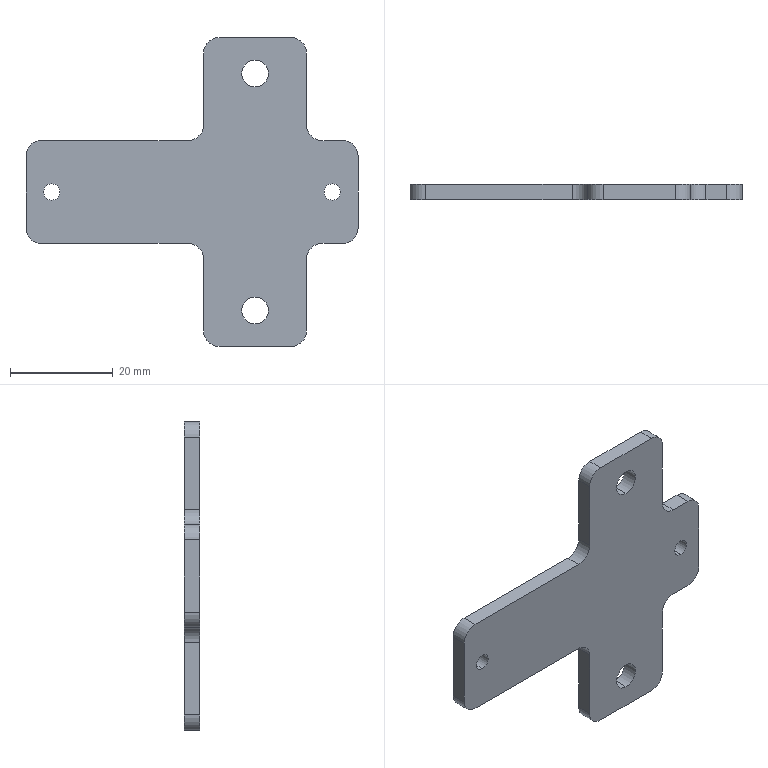Part | SolidWorks | features BaseBody 1 | 1 solid | 34 faces | box 64.5 x 3 x 60 mm | volume 6071 mm3 | cylinder 20 | plane 14 | commonest cylinder face diameters 6 x12 3.2 x4 5.2 x4
STEP:
#1=CARTESIAN_POINT('',(25.,0.,-31.6));
#2=VERTEX_POINT('',#1);
#3=CARTESIAN_POINT('',(25.,0.,-28.4));
#4=VERTEX_POINT('',#3);
#5=CARTESIAN_POINT('',(25.,0.,-30.));
#6=DIRECTION('',(0.,1.,0.));
#7=DIRECTION('',(0.,0.,1.));
#8=AXIS2_PLACEMENT_3D('',#5,#6,#7);
#9=CIRCLE('',#8,1.6);
#10=EDGE_CURVE('',#2,#4,#9,.T.);
#11=ORIENTED_EDGE('',*,*,#10,.F.);
#12=CARTESIAN_POINT('',(25.,3.,-31.6));
#13=VERTEX_POINT('',#12);
#14=CARTESIAN_POINT('',(25.,-39.878,-31.6));
#15=DIRECTION('',(0.,1.,0.));
#16=VECTOR('',#15,1000.);
#17=LINE('',#14,#16);
#18=EDGE_CURVE('',#2,#13,#17,.T.);
#19=ORIENTED_EDGE('',*,*,#18,.T.);
#20=CARTESIAN_POINT('',(25.,3.,-28.4));
#21=VERTEX_POINT('',#20);
#22=CARTESIAN_POINT('',(25.,3.,-30.));
#23=DIRECTION('',(0.,1.,0.));
#24=DIRECTION('',(0.,0.,1.));
#25=AXIS2_PLACEMENT_3D('',#22,#23,#24);
#26=CIRCLE('',#25,1.6);
#27=EDGE_CURVE('',#13,#21,#26,.T.);
#28=ORIENTED_EDGE('',*,*,#27,.T.);
#29=CARTESIAN_POINT('',(25.,-39.878,-28.4));
#30=DIRECTION('',(0.,1.,0.));
#31=VECTOR('',#30,1000.);
#32=LINE('',#29,#31);
#33=EDGE_CURVE('',#4,#21,#32,.T.);
#34=ORIENTED_EDGE('',*,*,#33,.F.);
#35=EDGE_LOOP('',(#11,#19,#28,#34));
#36=FACE_OUTER_BOUND('',#35,.T.);
#37=CARTESIAN_POINT('',(25.,-39.878,-30.));
#38=DIRECTION('',(0.,1.,0.));
#39=DIRECTION('',(0.,0.,1.));
#40=AXIS2_PLACEMENT_3D('',#37,#38,#39);
#41=CYLINDRICAL_SURFACE('',#40,1.6);
#42=ADVANCED_FACE('',(#36),#41,.F.);
#43=CARTESIAN_POINT('',(-29.5,0.,-31.6));
#44=VERTEX_POINT('',#43);
#45=CARTESIAN_POINT('',(-29.5,0.,-28.4));
#46=VERTEX_POINT('',#45);
#47=CARTESIAN_POINT('',(-29.5,0.,-30.));
#48=DIRECTION('',(0.,1.,0.));
#49=DIRECTION('',(0.,0.,1.));
#50=AXIS2_PLACEMENT_3D('',#47,#48,#49);
#51=CIRCLE('',#50,1.6);
#52=EDGE_CURVE('',#44,#46,#51,.T.);
#53=ORIENTED_EDGE('',*,*,#52,.F.);
#54=CARTESIAN_POINT('',(-29.5,3.,-31.6));
#55=VERTEX_POINT('',#54);
#56=CARTESIAN_POINT('',(-29.5,-39.878,-31.6));
#57=DIRECTION('',(0.,1.,0.));
#58=VECTOR('',#57,1000.);
#59=LINE('',#56,#58);
#60=EDGE_CURVE('',#44,#55,#59,.T.);
#61=ORIENTED_EDGE('',*,*,#60,.T.);
#62=CARTESIAN_POINT('',(-29.5,3.,-28.4));
#63=VERTEX_POINT('',#62);
#64=CARTESIAN_POINT('',(-29.5,3.,-30.));
#65=DIRECTION('',(0.,1.,0.));
#66=DIRECTION('',(0.,0.,1.));
#67=AXIS2_PLACEMENT_3D('',#64,#65,#66);
#68=CIRCLE('',#67,1.6);
#69=EDGE_CURVE('',#55,#63,#68,.T.);
#70=ORIENTED_EDGE('',*,*,#69,.T.);
#71=CARTESIAN_POINT('',(-29.5,-39.878,-28.4));
#72=DIRECTION('',(0.,1.,0.));
#73=VECTOR('',#72,1000.);
#74=LINE('',#71,#73);
#75=EDGE_CURVE('',#46,#63,#74,.T.);
#76=ORIENTED_EDGE('',*,*,#75,.F.);
#77=EDGE_LOOP('',(#53,#61,#70,#76));
#78=FACE_OUTER_BOUND('',#77,.T.);
#79=CARTESIAN_POINT('',(-29.5,-39.878,-30.));
#80=DIRECTION('',(0.,1.,0.));
#81=DIRECTION('',(0.,0.,1.));
#82=AXIS2_PLACEMENT_3D('',#79,#80,#81);
#83=CYLINDRICAL_SURFACE('',#82,1.6);
#84=ADVANCED_FACE('',(#78),#83,.F.);
#85=CARTESIAN_POINT('',(10.,3.,-55.6));
#86=VERTEX_POINT('',#85);
#87=CARTESIAN_POINT('',(10.,3.,-50.4));
#88=VERTEX_POINT('',#87);
#89=CARTESIAN_POINT('',(10.,3.,-53.));
#90=DIRECTION('',(0.,1.,0.));
#91=DIRECTION('',(0.,0.,-1.));
#92=AXIS2_PLACEMENT_3D('',#89,#90,#91);
#93=CIRCLE('',#92,2.6);
#94=EDGE_CURVE('',#86,#88,#93,.T.);
#95=ORIENTED_EDGE('',*,*,#94,.T.);
#96=CARTESIAN_POINT('',(10.,0.,-50.4));
#97=VERTEX_POINT('',#96);
#98=CARTESIAN_POINT('',(10.,3.,-50.4));
#99=DIRECTION('',(0.,-1.,0.));
#100=VECTOR('',#99,1000.);
#101=LINE('',#98,#100);
#102=EDGE_CURVE('',#88,#97,#101,.T.);
#103=ORIENTED_EDGE('',*,*,#102,.T.);
#104=CARTESIAN_POINT('',(10.,0.,-55.6));
#105=VERTEX_POINT('',#104);
#106=CARTESIAN_POINT('',(10.,0.,-53.));
#107=DIRECTION('',(0.,1.,0.));
#108=DIRECTION('',(0.,0.,-1.));
#109=AXIS2_PLACEMENT_3D('',#106,#107,#108);
#110=CIRCLE('',#109,2.6);
#111=EDGE_CURVE('',#105,#97,#110,.T.);
#112=ORIENTED_EDGE('',*,*,#111,.F.);
#113=CARTESIAN_POINT('',(10.,3.,-55.6));
#114=DIRECTION('',(0.,-1.,0.));
#115=VECTOR('',#114,1000.);
#116=LINE('',#113,#115);
#117=EDGE_CURVE('',#86,#105,#116,.T.);
#118=ORIENTED_EDGE('',*,*,#117,.F.);
#119=EDGE_LOOP('',(#95,#103,#112,#118));
#120=FACE_OUTER_BOUND('',#119,.T.);
#121=CARTESIAN_POINT('',(10.,3.,-53.));
#122=DIRECTION('',(0.,-1.,0.));
#123=DIRECTION('',(0.,0.,-1.));
#124=AXIS2_PLACEMENT_3D('',#121,#122,#123);
#125=CYLINDRICAL_SURFACE('',#124,2.6);
#126=ADVANCED_FACE('',(#120),#125,.F.);
#127=CARTESIAN_POINT('',(10.,3.,-9.6));
#128=VERTEX_POINT('',#127);
#129=CARTESIAN_POINT('',(10.,3.,-4.4));
#130=VERTEX_POINT('',#129);
#131=CARTESIAN_POINT('',(10.,3.,-7.));
#132=DIRECTION('',(0.,1.,0.));
#133=DIRECTION('',(0.,0.,-1.));
#134=AXIS2_PLACEMENT_3D('',#131,#132,#133);
#135=CIRCLE('',#134,2.6);
#136=EDGE_CURVE('',#128,#130,#135,.T.);
#137=ORIENTED_EDGE('',*,*,#136,.T.);
#138=CARTESIAN_POINT('',(10.,0.,-4.4));
#139=VERTEX_POINT('',#138);
#140=CARTESIAN_POINT('',(10.,3.,-4.4));
#141=DIRECTION('',(0.,-1.,0.));
#142=VECTOR('',#141,1000.);
#143=LINE('',#140,#142);
#144=EDGE_CURVE('',#130,#139,#143,.T.);
#145=ORIENTED_EDGE('',*,*,#144,.T.);
#146=CARTESIAN_POINT('',(10.,0.,-9.6));
#147=VERTEX_POINT('',#146);
#148=CARTESIAN_POINT('',(10.,0.,-7.));
#149=DIRECTION('',(0.,1.,0.));
#150=DIRECTION('',(0.,0.,-1.));
#151=AXIS2_PLACEMENT_3D('',#148,#149,#150);
#152=CIRCLE('',#151,2.6);
#153=EDGE_CURVE('',#147,#139,#152,.T.);
#154=ORIENTED_EDGE('',*,*,#153,.F.);
#155=CARTESIAN_POINT('',(10.,3.,-9.6));
#156=DIRECTION('',(0.,-1.,0.));
#157=VECTOR('',#156,1000.);
#158=LINE('',#155,#157);
#159=EDGE_CURVE('',#128,#147,#158,.T.);
#160=ORIENTED_EDGE('',*,*,#159,.F.);
#161=EDGE_LOOP('',(#137,#145,#154,#160));
#162=FACE_OUTER_BOUND('',#161,.T.);
#163=CARTESIAN_POINT('',(10.,3.,-7.));
#164=DIRECTION('',(0.,-1.,0.));
#165=DIRECTION('',(0.,0.,-1.));
#166=AXIS2_PLACEMENT_3D('',#163,#164,#165);
#167=CYLINDRICAL_SURFACE('',#166,2.6);
#168=ADVANCED_FACE('',(#162),#167,.F.);
#169=CARTESIAN_POINT('',(25.,3.,-30.));
#170=DIRECTION('',(0.,1.,0.));
#171=DIRECTION('',(0.,0.,1.));
#172=AXIS2_PLACEMENT_3D('',#169,#170,#171);
#173=CIRCLE('',#172,1.6);
#174=EDGE_CURVE('',#21,#13,#173,.T.);
#175=ORIENTED_EDGE('',*,*,#174,.F.);
#176=ORIENTED_EDGE('',*,*,#27,.F.);
#177=EDGE_LOOP('',(#175,#176));
#178=FACE_BOUND('',#177,.T.);
#179=CARTESIAN_POINT('',(-29.5,3.,-30.));
#180=DIRECTION('',(0.,1.,0.));
#181=DIRECTION('',(0.,0.,1.));
#182=AXIS2_PLACEMENT_3D('',#179,#180,#181);
#183=CIRCLE('',#182,1.6);
#184=EDGE_CURVE('',#63,#55,#183,.T.);
#185=ORIENTED_EDGE('',*,*,#184,.F.);
#186=ORIENTED_EDGE('',*,*,#69,.F.);
#187=EDGE_LOOP('',(#185,#186));
#188=FACE_BOUND('',#187,.T.);
#189=ORIENTED_EDGE('',*,*,#94,.F.);
#190=CARTESIAN_POINT('',(10.,3.,-53.));
#191=DIRECTION('',(0.,1.,0.));
#192=DIRECTION('',(0.,0.,-1.));
#193=AXIS2_PLACEMENT_3D('',#190,#191,#192);
#194=CIRCLE('',#193,2.6);
#195=EDGE_CURVE('',#88,#86,#194,.T.);
#196=ORIENTED_EDGE('',*,*,#195,.F.);
#197=EDGE_LOOP('',(#189,#196));
#198=FACE_BOUND('',#197,.T.);
#199=ORIENTED_EDGE('',*,*,#136,.F.);
#200=CARTESIAN_POINT('',(10.,3.,-7.));
#201=DIRECTION('',(0.,1.,0.));
#202=DIRECTION('',(0.,0.,-1.));
#203=AXIS2_PLACEMENT_3D('',#200,#201,#202);
#204=CIRCLE('',#203,2.6);
#205=EDGE_CURVE('',#130,#128,#204,.T.);
#206=ORIENTED_EDGE('',*,*,#205,.F.);
#207=EDGE_LOOP('',(#199,#206));
#208=FACE_BOUND('',#207,.T.);
#209=CARTESIAN_POINT('',(-31.5,3.,-20.));
#210=VERTEX_POINT('',#209);
#211=CARTESIAN_POINT('',(-34.5,3.,-23.));
#212=VERTEX_POINT('',#211);
#213=CARTESIAN_POINT('',(-31.5,3.,-23.));
#214=DIRECTION('',(0.,-1.,0.));
#215=DIRECTION('',(0.,0.,1.));
#216=AXIS2_PLACEMENT_3D('',#213,#214,#215);
#217=CIRCLE('',#216,3.);
#218=EDGE_CURVE('',#210,#212,#217,.T.);
#219=ORIENTED_EDGE('',*,*,#218,.F.);
#220=CARTESIAN_POINT('',(-3.,3.,-20.));
#221=VERTEX_POINT('',#220);
#222=CARTESIAN_POINT('',(0.,3.,-20.));
#223=DIRECTION('',(-1.,0.,0.));
#224=VECTOR('',#223,1000.);
#225=LINE('',#222,#224);
#226=EDGE_CURVE('',#221,#210,#225,.T.);
#227=ORIENTED_EDGE('',*,*,#226,.F.);
#228=CARTESIAN_POINT('',(0.,3.,-17.));
#229=VERTEX_POINT('',#228);
#230=CARTESIAN_POINT('',(-3.,3.,-17.));
#231=DIRECTION('',(0.,1.,0.));
#232=DIRECTION('',(0.,0.,1.));
#233=AXIS2_PLACEMENT_3D('',#230,#231,#232);
#234=CIRCLE('',#233,3.);
#235=EDGE_CURVE('',#229,#221,#234,.T.);
#236=ORIENTED_EDGE('',*,*,#235,.F.);
#237=CARTESIAN_POINT('',(0.,3.,-3.));
#238=VERTEX_POINT('',#237);
#239=CARTESIAN_POINT('',(0.,3.,0.));
#240=DIRECTION('',(0.,0.,-1.));
#241=VECTOR('',#240,1000.);
#242=LINE('',#239,#241);
#243=EDGE_CURVE('',#238,#229,#242,.T.);
#244=ORIENTED_EDGE('',*,*,#243,.F.);
#245=CARTESIAN_POINT('',(3.,3.,0.));
#246=VERTEX_POINT('',#245);
#247=CARTESIAN_POINT('',(3.,3.,-3.));
#248=DIRECTION('',(0.,-1.,0.));
#249=DIRECTION('',(0.,0.,-1.));
#250=AXIS2_PLACEMENT_3D('',#247,#248,#249);
#251=CIRCLE('',#250,3.);
#252=EDGE_CURVE('',#246,#238,#251,.T.);
#253=ORIENTED_EDGE('',*,*,#252,.F.);
#254=CARTESIAN_POINT('',(17.,3.,0.));
#255=VERTEX_POINT('',#254);
#256=CARTESIAN_POINT('',(0.,3.,0.));
#257=DIRECTION('',(-1.,0.,0.));
#258=VECTOR('',#257,1000.);
#259=LINE('',#256,#258);
#260=EDGE_CURVE('',#255,#246,#259,.T.);
#261=ORIENTED_EDGE('',*,*,#260,.F.);
#262=CARTESIAN_POINT('',(20.,3.,-3.));
#263=VERTEX_POINT('',#262);
#264=CARTESIAN_POINT('',(17.,3.,-3.));
#265=DIRECTION('',(0.,-1.,0.));
#266=DIRECTION('',(0.,0.,-1.));
#267=AXIS2_PLACEMENT_3D('',#264,#265,#266);
#268=CIRCLE('',#267,3.);
#269=EDGE_CURVE('',#263,#255,#268,.T.);
#270=ORIENTED_EDGE('',*,*,#269,.F.);
#271=CARTESIAN_POINT('',(20.,3.,-17.));
#272=VERTEX_POINT('',#271);
#273=CARTESIAN_POINT('',(20.,3.,0.));
#274=DIRECTION('',(0.,0.,1.));
#275=VECTOR('',#274,1000.);
#276=LINE('',#273,#275);
#277=EDGE_CURVE('',#272,#263,#276,.T.);
#278=ORIENTED_EDGE('',*,*,#277,.F.);
#279=CARTESIAN_POINT('',(23.,3.,-20.));
#280=VERTEX_POINT('',#279);
#281=CARTESIAN_POINT('',(23.,3.,-17.));
#282=DIRECTION('',(0.,1.,0.));
#283=DIRECTION('',(0.,0.,1.));
#284=AXIS2_PLACEMENT_3D('',#281,#282,#283);
#285=CIRCLE('',#284,3.);
#286=EDGE_CURVE('',#280,#272,#285,.T.);
#287=ORIENTED_EDGE('',*,*,#286,.F.);
#288=CARTESIAN_POINT('',(27.,3.,-20.));
#289=VERTEX_POINT('',#288);
#290=CARTESIAN_POINT('',(0.,3.,-20.));
#291=DIRECTION('',(-1.,0.,0.));
#292=VECTOR('',#291,1000.);
#293=LINE('',#290,#292);
#294=EDGE_CURVE('',#289,#280,#293,.T.);
#295=ORIENTED_EDGE('',*,*,#294,.F.);
#296=CARTESIAN_POINT('',(30.,3.,-23.));
#297=VERTEX_POINT('',#296);
#298=CARTESIAN_POINT('',(27.,3.,-23.));
#299=DIRECTION('',(0.,-1.,0.));
#300=DIRECTION('',(0.,0.,1.));
#301=AXIS2_PLACEMENT_3D('',#298,#299,#300);
#302=CIRCLE('',#301,3.);
#303=EDGE_CURVE('',#297,#289,#302,.T.);
#304=ORIENTED_EDGE('',*,*,#303,.F.);
#305=CARTESIAN_POINT('',(30.,3.,-37.));
#306=VERTEX_POINT('',#305);
#307=CARTESIAN_POINT('',(30.,3.,0.));
#308=DIRECTION('',(0.,0.,1.));
#309=VECTOR('',#308,1000.);
#310=LINE('',#307,#309);
#311=EDGE_CURVE('',#306,#297,#310,.T.);
#312=ORIENTED_EDGE('',*,*,#311,.F.);
#313=CARTESIAN_POINT('',(27.,3.,-40.));
#314=VERTEX_POINT('',#313);
#315=CARTESIAN_POINT('',(27.,3.,-37.));
#316=DIRECTION('',(0.,-1.,0.));
#317=DIRECTION('',(0.,0.,1.));
#318=AXIS2_PLACEMENT_3D('',#315,#316,#317);
#319=CIRCLE('',#318,3.);
#320=EDGE_CURVE('',#314,#306,#319,.T.);
#321=ORIENTED_EDGE('',*,*,#320,.F.);
#322=CARTESIAN_POINT('',(23.,3.,-40.));
#323=VERTEX_POINT('',#322);
#324=CARTESIAN_POINT('',(0.,3.,-40.));
#325=DIRECTION('',(1.,0.,0.));
#326=VECTOR('',#325,1000.);
#327=LINE('',#324,#326);
#328=EDGE_CURVE('',#323,#314,#327,.T.);
#329=ORIENTED_EDGE('',*,*,#328,.F.);
#330=CARTESIAN_POINT('',(20.,3.,-43.));
#331=VERTEX_POINT('',#330);
#332=CARTESIAN_POINT('',(23.,3.,-43.));
#333=DIRECTION('',(0.,1.,0.));
#334=DIRECTION('',(0.,0.,1.));
#335=AXIS2_PLACEMENT_3D('',#332,#333,#334);
#336=CIRCLE('',#335,3.);
#337=EDGE_CURVE('',#331,#323,#336,.T.);
#338=ORIENTED_EDGE('',*,*,#337,.F.);
#339=CARTESIAN_POINT('',(20.,3.,-57.));
#340=VERTEX_POINT('',#339);
#341=CARTESIAN_POINT('',(20.,3.,0.));
#342=DIRECTION('',(0.,0.,1.));
#343=VECTOR('',#342,1000.);
#344=LINE('',#341,#343);
#345=EDGE_CURVE('',#340,#331,#344,.T.);
#346=ORIENTED_EDGE('',*,*,#345,.F.);
#347=CARTESIAN_POINT('',(17.,3.,-60.));
#348=VERTEX_POINT('',#347);
#349=CARTESIAN_POINT('',(17.,3.,-57.));
#350=DIRECTION('',(0.,-1.,0.));
#351=DIRECTION('',(0.,0.,-1.));
#352=AXIS2_PLACEMENT_3D('',#349,#350,#351);
#353=CIRCLE('',#352,3.);
#354=EDGE_CURVE('',#348,#340,#353,.T.);
#355=ORIENTED_EDGE('',*,*,#354,.F.);
#356=CARTESIAN_POINT('',(3.,3.,-60.));
#357=VERTEX_POINT('',#356);
#358=CARTESIAN_POINT('',(0.,3.,-60.));
#359=DIRECTION('',(1.,0.,0.));
#360=VECTOR('',#359,1000.);
#361=LINE('',#358,#360);
#362=EDGE_CURVE('',#357,#348,#361,.T.);
#363=ORIENTED_EDGE('',*,*,#362,.F.);
#364=CARTESIAN_POINT('',(0.,3.,-57.));
#365=VERTEX_POINT('',#364);
#366=CARTESIAN_POINT('',(3.,3.,-57.));
#367=DIRECTION('',(0.,-1.,0.));
#368=DIRECTION('',(0.,0.,-1.));
#369=AXIS2_PLACEMENT_3D('',#366,#367,#368);
#370=CIRCLE('',#369,3.);
#371=EDGE_CURVE('',#365,#357,#370,.T.);
#372=ORIENTED_EDGE('',*,*,#371,.F.);
#373=CARTESIAN_POINT('',(0.,3.,-43.));
#374=VERTEX_POINT('',#373);
#375=CARTESIAN_POINT('',(0.,3.,0.));
#376=DIRECTION('',(0.,0.,-1.));
#377=VECTOR('',#376,1000.);
#378=LINE('',#375,#377);
#379=EDGE_CURVE('',#374,#365,#378,.T.);
#380=ORIENTED_EDGE('',*,*,#379,.F.);
#381=CARTESIAN_POINT('',(-3.,3.,-40.));
#382=VERTEX_POINT('',#381);
#383=CARTESIAN_POINT('',(-3.,3.,-43.));
#384=DIRECTION('',(0.,1.,0.));
#385=DIRECTION('',(0.,0.,1.));
#386=AXIS2_PLACEMENT_3D('',#383,#384,#385);
#387=CIRCLE('',#386,3.);
#388=EDGE_CURVE('',#382,#374,#387,.T.);
#389=ORIENTED_EDGE('',*,*,#388,.F.);
#390=CARTESIAN_POINT('',(-31.5,3.,-40.));
#391=VERTEX_POINT('',#390);
#392=CARTESIAN_POINT('',(0.,3.,-40.));
#393=DIRECTION('',(1.,0.,0.));
#394=VECTOR('',#393,1000.);
#395=LINE('',#392,#394);
#396=EDGE_CURVE('',#391,#382,#395,.T.);
#397=ORIENTED_EDGE('',*,*,#396,.F.);
#398=CARTESIAN_POINT('',(-34.5,3.,-37.));
#399=VERTEX_POINT('',#398);
#400=CARTESIAN_POINT('',(-31.5,3.,-37.));
#401=DIRECTION('',(0.,-1.,0.));
#402=DIRECTION('',(0.,0.,1.));
#403=AXIS2_PLACEMENT_3D('',#400,#401,#402);
#404=CIRCLE('',#403,3.);
#405=EDGE_CURVE('',#399,#391,#404,.T.);
#406=ORIENTED_EDGE('',*,*,#405,.F.);
#407=CARTESIAN_POINT('',(-34.5,3.,0.));
#408=DIRECTION('',(0.,0.,-1.));
#409=VECTOR('',#408,1000.);
#410=LINE('',#407,#409);
#411=EDGE_CURVE('',#212,#399,#410,.T.);
#412=ORIENTED_EDGE('',*,*,#411,.F.);
#413=EDGE_LOOP('',(#219,#227,#236,#244,#253,#261,#270,#278,#287,#295,#304,#312,#321,#329,#338,#346,#355,#363,#372,#380,#389,#397,#406,#412));
#414=FACE_OUTER_BOUND('',#413,.T.);
#415=CARTESIAN_POINT('',(0.,3.,0.));
#416=DIRECTION('',(0.,-1.,0.));
#417=DIRECTION('',(0.,0.,-1.));
#418=AXIS2_PLACEMENT_3D('',#415,#416,#417);
#419=PLANE('',#418);
#420=ADVANCED_FACE('',(#178,#188,#198,#208,#414),#419,.F.);
#421=ORIENTED_EDGE('',*,*,#18,.F.);
#422=CARTESIAN_POINT('',(25.,0.,-30.));
#423=DIRECTION('',(0.,1.,0.));
#424=DIRECTION('',(0.,0.,1.));
#425=AXIS2_PLACEMENT_3D('',#422,#423,#424);
#426=CIRCLE('',#425,1.6);
#427=EDGE_CURVE('',#4,#2,#426,.T.);
#428=ORIENTED_EDGE('',*,*,#427,.F.);
#429=ORIENTED_EDGE('',*,*,#33,.T.);
#430=ORIENTED_EDGE('',*,*,#174,.T.);
#431=EDGE_LOOP('',(#421,#428,#429,#430));
#432=FACE_OUTER_BOUND('',#431,.T.);
#433=CARTESIAN_POINT('',(25.,-39.878,-30.));
#434=DIRECTION('',(0.,1.,0.));
#435=DIRECTION('',(0.,0.,1.));
#436=AXIS2_PLACEMENT_3D('',#433,#434,#435);
#437=CYLINDRICAL_SURFACE('',#436,1.6);
#438=ADVANCED_FACE('',(#432),#437,.F.);
#439=ORIENTED_EDGE('',*,*,#60,.F.);
#440=CARTESIAN_POINT('',(-29.5,0.,-30.));
#441=DIRECTION('',(0.,1.,0.));
#442=DIRECTION('',(0.,0.,1.));
#443=AXIS2_PLACEMENT_3D('',#440,#441,#442);
#444=CIRCLE('',#443,1.6);
#445=EDGE_CURVE('',#46,#44,#444,.T.);
#446=ORIENTED_EDGE('',*,*,#445,.F.);
#447=ORIENTED_EDGE('',*,*,#75,.T.);
#448=ORIENTED_EDGE('',*,*,#184,.T.);
#449=EDGE_LOOP('',(#439,#446,#447,#448));
#450=FACE_OUTER_BOUND('',#449,.T.);
#451=CARTESIAN_POINT('',(-29.5,-39.878,-30.));
#452=DIRECTION('',(0.,1.,0.));
#453=DIRECTION('',(0.,0.,1.));
#454=AXIS2_PLACEMENT_3D('',#451,#452,#453);
#455=CYLINDRICAL_SURFACE('',#454,1.6);
#456=ADVANCED_FACE('',(#450),#455,.F.);
#457=ORIENTED_EDGE('',*,*,#102,.F.);
#458=ORIENTED_EDGE('',*,*,#195,.T.);
#459=ORIENTED_EDGE('',*,*,#117,.T.);
#460=CARTESIAN_POINT('',(10.,0.,-53.));
#461=DIRECTION('',(0.,1.,0.));
#462=DIRECTION('',(0.,0.,-1.));
#463=AXIS2_PLACEMENT_3D('',#460,#461,#462);
#464=CIRCLE('',#463,2.6);
#465=EDGE_CURVE('',#97,#105,#464,.T.);
#466=ORIENTED_EDGE('',*,*,#465,.F.);
#467=EDGE_LOOP('',(#457,#458,#459,#466));
#468=FACE_OUTER_BOUND('',#467,.T.);
#469=CARTESIAN_POINT('',(10.,3.,-53.));
#470=DIRECTION('',(0.,-1.,0.));
#471=DIRECTION('',(0.,0.,-1.));
#472=AXIS2_PLACEMENT_3D('',#469,#470,#471);
#473=CYLINDRICAL_SURFACE('',#472,2.6);
#474=ADVANCED_FACE('',(#468),#473,.F.);
#475=ORIENTED_EDGE('',*,*,#144,.F.);
#476=ORIENTED_EDGE('',*,*,#205,.T.);
#477=ORIENTED_EDGE('',*,*,#159,.T.);
#478=CARTESIAN_POINT('',(10.,0.,-7.));
#479=DIRECTION('',(0.,1.,0.));
#480=DIRECTION('',(0.,0.,-1.));
#481=AXIS2_PLACEMENT_3D('',#478,#479,#480);
#482=CIRCLE('',#481,2.6);
#483=EDGE_CURVE('',#139,#147,#482,.T.);
#484=ORIENTED_EDGE('',*,*,#483,.F.);
#485=EDGE_LOOP('',(#475,#476,#477,#484));
#486=FACE_OUTER_BOUND('',#485,.T.);
#487=CARTESIAN_POINT('',(10.,3.,-7.));
#488=DIRECTION('',(0.,-1.,0.));
#489=DIRECTION('',(0.,0.,-1.));
#490=AXIS2_PLACEMENT_3D('',#487,#488,#489);
#491=CYLINDRICAL_SURFACE('',#490,2.6);
#492=ADVANCED_FACE('',(#486),#491,.F.);
#493=ORIENTED_EDGE('',*,*,#411,.T.);
#494=CARTESIAN_POINT('',(-34.5,0.,-37.));
#495=VERTEX_POINT('',#494);
#496=CARTESIAN_POINT('',(-34.5,-39.878,-37.));
#497=DIRECTION('',(0.,-1.,0.));
#498=VECTOR('',#497,1000.);
#499=LINE('',#496,#498);
#500=EDGE_CURVE('',#399,#495,#499,.T.);
#501=ORIENTED_EDGE('',*,*,#500,.T.);
#502=CARTESIAN_POINT('',(-34.5,0.,-23.));
#503=VERTEX_POINT('',#502);
#504=CARTESIAN_POINT('',(-34.5,0.,-20.));
#505=DIRECTION('',(0.,0.,1.));
#506=VECTOR('',#505,1000.);
#507=LINE('',#504,#506);
#508=EDGE_CURVE('',#495,#503,#507,.T.);
#509=ORIENTED_EDGE('',*,*,#508,.T.);
#510=CARTESIAN_POINT('',(-34.5,-39.878,-23.));
#511=DIRECTION('',(0.,1.,0.));
#512=VECTOR('',#511,1000.);
#513=LINE('',#510,#512);
#514=EDGE_CURVE('',#503,#212,#513,.T.);
#515=ORIENTED_EDGE('',*,*,#514,.T.);
#516=EDGE_LOOP('',(#493,#501,#509,#515));
#517=FACE_OUTER_BOUND('',#516,.T.);
#518=CARTESIAN_POINT('',(-34.5,-39.878,-20.));
#519=DIRECTION('',(-1.,0.,0.));
#520=DIRECTION('',(0.,0.,1.));
#521=AXIS2_PLACEMENT_3D('',#518,#519,#520);
#522=PLANE('',#521);
#523=ADVANCED_FACE('',(#517),#522,.T.);
#524=ORIENTED_EDGE('',*,*,#218,.T.);
#525=ORIENTED_EDGE('',*,*,#514,.F.);
#526=CARTESIAN_POINT('',(-31.5,0.,-20.));
#527=VERTEX_POINT('',#526);
#528=CARTESIAN_POINT('',(-31.5,0.,-23.));
#529=DIRECTION('',(0.,1.,0.));
#530=DIRECTION('',(0.,0.,1.));
#531=AXIS2_PLACEMENT_3D('',#528,#529,#530);
#532=CIRCLE('',#531,3.);
#533=EDGE_CURVE('',#503,#527,#532,.T.);
#534=ORIENTED_EDGE('',*,*,#533,.T.);
#535=CARTESIAN_POINT('',(-31.5,-39.878,-20.));
#536=DIRECTION('',(0.,1.,0.));
#537=VECTOR('',#536,1000.);
#538=LINE('',#535,#537);
#539=EDGE_CURVE('',#527,#210,#538,.T.);
#540=ORIENTED_EDGE('',*,*,#539,.T.);
#541=EDGE_LOOP('',(#524,#525,#534,#540));
#542=FACE_OUTER_BOUND('',#541,.T.);
#543=CARTESIAN_POINT('',(-31.5,-39.878,-23.));
#544=DIRECTION('',(0.,1.,0.));
#545=DIRECTION('',(0.,0.,1.));
#546=AXIS2_PLACEMENT_3D('',#543,#544,#545);
#547=CYLINDRICAL_SURFACE('',#546,3.);
#548=ADVANCED_FACE('',(#542),#547,.T.);
#549=CARTESIAN_POINT('',(-3.,0.,-20.));
#550=VERTEX_POINT('',#549);
#551=CARTESIAN_POINT('',(0.,0.,-20.));
#552=DIRECTION('',(1.,0.,0.));
#553=VECTOR('',#552,1000.);
#554=LINE('',#551,#553);
#555=EDGE_CURVE('',#527,#550,#554,.T.);
#556=ORIENTED_EDGE('',*,*,#555,.T.);
#557=CARTESIAN_POINT('',(-3.,-39.878,-20.));
#558=DIRECTION('',(0.,1.,0.));
#559=VECTOR('',#558,1000.);
#560=LINE('',#557,#559);
#561=EDGE_CURVE('',#550,#221,#560,.T.);
#562=ORIENTED_EDGE('',*,*,#561,.T.);
#563=ORIENTED_EDGE('',*,*,#226,.T.);
#564=ORIENTED_EDGE('',*,*,#539,.F.);
#565=EDGE_LOOP('',(#556,#562,#563,#564));
#566=FACE_OUTER_BOUND('',#565,.T.);
#567=CARTESIAN_POINT('',(0.,-39.878,-20.));
#568=DIRECTION('',(0.,0.,1.));
#569=DIRECTION('',(1.,0.,0.));
#570=AXIS2_PLACEMENT_3D('',#567,#568,#569);
#571=PLANE('',#570);
#572=ADVANCED_FACE('',(#566),#571,.T.);
#573=CARTESIAN_POINT('',(0.,0.,-17.));
#574=VERTEX_POINT('',#573);
#575=CARTESIAN_POINT('',(0.,-39.878,-17.));
#576=DIRECTION('',(0.,-1.,0.));
#577=VECTOR('',#576,1000.);
#578=LINE('',#575,#577);
#579=EDGE_CURVE('',#229,#574,#578,.T.);
#580=ORIENTED_EDGE('',*,*,#579,.F.);
#581=ORIENTED_EDGE('',*,*,#235,.T.);
#582=ORIENTED_EDGE('',*,*,#561,.F.);
#583=CARTESIAN_POINT('',(-3.,0.,-17.));
#584=DIRECTION('',(0.,1.,0.));
#585=DIRECTION('',(0.,0.,1.));
#586=AXIS2_PLACEMENT_3D('',#583,#584,#585);
#587=CIRCLE('',#586,3.);
#588=EDGE_CURVE('',#574,#550,#587,.T.);
#589=ORIENTED_EDGE('',*,*,#588,.F.);
#590=EDGE_LOOP('',(#580,#581,#582,#589));
#591=FACE_OUTER_BOUND('',#590,.T.);
#592=CARTESIAN_POINT('',(-3.,-39.878,-17.));
#593=DIRECTION('',(0.,1.,0.));
#594=DIRECTION('',(0.,0.,1.));
#595=AXIS2_PLACEMENT_3D('',#592,#593,#594);
#596=CYLINDRICAL_SURFACE('',#595,3.);
#597=ADVANCED_FACE('',(#591),#596,.F.);
#598=ORIENTED_EDGE('',*,*,#579,.T.);
#599=CARTESIAN_POINT('',(0.,0.,-3.));
#600=VERTEX_POINT('',#599);
#601=CARTESIAN_POINT('',(0.,0.,0.));
#602=DIRECTION('',(0.,0.,-1.));
#603=VECTOR('',#602,1000.);
#604=LINE('',#601,#603);
#605=EDGE_CURVE('',#600,#574,#604,.T.);
#606=ORIENTED_EDGE('',*,*,#605,.F.);
#607=CARTESIAN_POINT('',(0.,3.,-3.));
#608=DIRECTION('',(0.,-1.,0.));
#609=VECTOR('',#608,1000.);
#610=LINE('',#607,#609);
#611=EDGE_CURVE('',#238,#600,#610,.T.);
#612=ORIENTED_EDGE('',*,*,#611,.F.);
#613=ORIENTED_EDGE('',*,*,#243,.T.);
#614=EDGE_LOOP('',(#598,#606,#612,#613));
#615=FACE_OUTER_BOUND('',#614,.T.);
#616=CARTESIAN_POINT('',(0.,3.,0.));
#617=DIRECTION('',(1.,0.,0.));
#618=DIRECTION('',(0.,0.,-1.));
#619=AXIS2_PLACEMENT_3D('',#616,#617,#618);
#620=PLANE('',#619);
#621=ADVANCED_FACE('',(#615),#620,.F.);
#622=CARTESIAN_POINT('',(3.,0.,0.));
#623=VERTEX_POINT('',#622);
#624=CARTESIAN_POINT('',(3.,0.,-3.));
#625=DIRECTION('',(0.,1.,0.));
#626=DIRECTION('',(0.,0.,-1.));
#627=AXIS2_PLACEMENT_3D('',#624,#625,#626);
#628=CIRCLE('',#627,3.);
#629=EDGE_CURVE('',#600,#623,#628,.T.);
#630=ORIENTED_EDGE('',*,*,#629,.T.);
#631=CARTESIAN_POINT('',(3.,3.,0.));
#632=DIRECTION('',(0.,1.,0.));
#633=VECTOR('',#632,1000.);
#634=LINE('',#631,#633);
#635=EDGE_CURVE('',#623,#246,#634,.T.);
#636=ORIENTED_EDGE('',*,*,#635,.T.);
#637=ORIENTED_EDGE('',*,*,#252,.T.);
#638=ORIENTED_EDGE('',*,*,#611,.T.);
#639=EDGE_LOOP('',(#630,#636,#637,#638));
#640=FACE_OUTER_BOUND('',#639,.T.);
#641=CARTESIAN_POINT('',(3.,3.,-3.));
#642=DIRECTION('',(0.,-1.,0.));
#643=DIRECTION('',(0.,0.,-1.));
#644=AXIS2_PLACEMENT_3D('',#641,#642,#643);
#645=CYLINDRICAL_SURFACE('',#644,3.);
#646=ADVANCED_FACE('',(#640),#645,.T.);
#647=CARTESIAN_POINT('',(17.,0.,0.));
#648=VERTEX_POINT('',#647);
#649=CARTESIAN_POINT('',(17.,3.,0.));
#650=DIRECTION('',(0.,-1.,0.));
#651=VECTOR('',#650,1000.);
#652=LINE('',#649,#651);
#653=EDGE_CURVE('',#255,#648,#652,.T.);
#654=ORIENTED_EDGE('',*,*,#653,.F.);
#655=ORIENTED_EDGE('',*,*,#260,.T.);
#656=ORIENTED_EDGE('',*,*,#635,.F.);
#657=CARTESIAN_POINT('',(0.,0.,0.));
#658=DIRECTION('',(-1.,0.,0.));
#659=VECTOR('',#658,1000.);
#660=LINE('',#657,#659);
#661=EDGE_CURVE('',#648,#623,#660,.T.);
#662=ORIENTED_EDGE('',*,*,#661,.F.);
#663=EDGE_LOOP('',(#654,#655,#656,#662));
#664=FACE_OUTER_BOUND('',#663,.T.);
#665=CARTESIAN_POINT('',(0.,3.,0.));
#666=DIRECTION('',(0.,0.,-1.));
#667=DIRECTION('',(-1.,0.,0.));
#668=AXIS2_PLACEMENT_3D('',#665,#666,#667);
#669=PLANE('',#668);
#670=ADVANCED_FACE('',(#664),#669,.F.);
#671=CARTESIAN_POINT('',(20.,0.,-3.));
#672=VERTEX_POINT('',#671);
#673=CARTESIAN_POINT('',(17.,0.,-3.));
#674=DIRECTION('',(0.,1.,0.));
#675=DIRECTION('',(0.,0.,-1.));
#676=AXIS2_PLACEMENT_3D('',#673,#674,#675);
#677=CIRCLE('',#676,3.);
#678=EDGE_CURVE('',#648,#672,#677,.T.);
#679=ORIENTED_EDGE('',*,*,#678,.T.);
#680=CARTESIAN_POINT('',(20.,3.,-3.));
#681=DIRECTION('',(0.,1.,0.));
#682=VECTOR('',#681,1000.);
#683=LINE('',#680,#682);
#684=EDGE_CURVE('',#672,#263,#683,.T.);
#685=ORIENTED_EDGE('',*,*,#684,.T.);
#686=ORIENTED_EDGE('',*,*,#269,.T.);
#687=ORIENTED_EDGE('',*,*,#653,.T.);
#688=EDGE_LOOP('',(#679,#685,#686,#687));
#689=FACE_OUTER_BOUND('',#688,.T.);
#690=CARTESIAN_POINT('',(17.,3.,-3.));
#691=DIRECTION('',(0.,-1.,0.));
#692=DIRECTION('',(0.,0.,-1.));
#693=AXIS2_PLACEMENT_3D('',#690,#691,#692);
#694=CYLINDRICAL_SURFACE('',#693,3.);
#695=ADVANCED_FACE('',(#689),#694,.T.);
#696=CARTESIAN_POINT('',(20.,0.,-17.));
#697=VERTEX_POINT('',#696);
#698=CARTESIAN_POINT('',(20.,3.,-17.));
#699=DIRECTION('',(0.,-1.,0.));
#700=VECTOR('',#699,1000.);
#701=LINE('',#698,#700);
#702=EDGE_CURVE('',#272,#697,#701,.T.);
#703=ORIENTED_EDGE('',*,*,#702,.F.);
#704=ORIENTED_EDGE('',*,*,#277,.T.);
#705=ORIENTED_EDGE('',*,*,#684,.F.);
#706=CARTESIAN_POINT('',(20.,0.,0.));
#707=DIRECTION('',(0.,0.,1.));
#708=VECTOR('',#707,1000.);
#709=LINE('',#706,#708);
#710=EDGE_CURVE('',#697,#672,#709,.T.);
#711=ORIENTED_EDGE('',*,*,#710,.F.);
#712=EDGE_LOOP('',(#703,#704,#705,#711));
#713=FACE_OUTER_BOUND('',#712,.T.);
#714=CARTESIAN_POINT('',(20.,3.,0.));
#715=DIRECTION('',(-1.,0.,0.));
#716=DIRECTION('',(0.,0.,1.));
#717=AXIS2_PLACEMENT_3D('',#714,#715,#716);
#718=PLANE('',#717);
#719=ADVANCED_FACE('',(#713),#718,.F.);
#720=CARTESIAN_POINT('',(23.,0.,-20.));
#721=VERTEX_POINT('',#720);
#722=CARTESIAN_POINT('',(23.,3.,-20.));
#723=DIRECTION('',(0.,-1.,0.));
#724=VECTOR('',#723,1000.);
#725=LINE('',#722,#724);
#726=EDGE_CURVE('',#280,#721,#725,.T.);
#727=ORIENTED_EDGE('',*,*,#726,.F.);
#728=ORIENTED_EDGE('',*,*,#286,.T.);
#729=ORIENTED_EDGE('',*,*,#702,.T.);
#730=CARTESIAN_POINT('',(23.,0.,-17.));
#731=DIRECTION('',(0.,1.,0.));
#732=DIRECTION('',(0.,0.,1.));
#733=AXIS2_PLACEMENT_3D('',#730,#731,#732);
#734=CIRCLE('',#733,3.);
#735=EDGE_CURVE('',#721,#697,#734,.T.);
#736=ORIENTED_EDGE('',*,*,#735,.F.);
#737=EDGE_LOOP('',(#727,#728,#729,#736));
#738=FACE_OUTER_BOUND('',#737,.T.);
#739=CARTESIAN_POINT('',(23.,3.,-17.));
#740=DIRECTION('',(0.,1.,0.));
#741=DIRECTION('',(0.,0.,1.));
#742=AXIS2_PLACEMENT_3D('',#739,#740,#741);
#743=CYLINDRICAL_SURFACE('',#742,3.);
#744=ADVANCED_FACE('',(#738),#743,.F.);
#745=CARTESIAN_POINT('',(27.,0.,-20.));
#746=VERTEX_POINT('',#745);
#747=CARTESIAN_POINT('',(20.,0.,-20.));
#748=DIRECTION('',(1.,0.,0.));
#749=VECTOR('',#748,1000.);
#750=LINE('',#747,#749);
#751=EDGE_CURVE('',#721,#746,#750,.T.);
#752=ORIENTED_EDGE('',*,*,#751,.T.);
#753=CARTESIAN_POINT('',(27.,-39.878,-20.));
#754=DIRECTION('',(0.,1.,0.));
#755=VECTOR('',#754,1000.);
#756=LINE('',#753,#755);
#757=EDGE_CURVE('',#746,#289,#756,.T.);
#758=ORIENTED_EDGE('',*,*,#757,.T.);
#759=ORIENTED_EDGE('',*,*,#294,.T.);
#760=ORIENTED_EDGE('',*,*,#726,.T.);
#761=EDGE_LOOP('',(#752,#758,#759,#760));
#762=FACE_OUTER_BOUND('',#761,.T.);
#763=CARTESIAN_POINT('',(20.,-39.878,-20.));
#764=DIRECTION('',(0.,0.,1.));
#765=DIRECTION('',(1.,0.,0.));
#766=AXIS2_PLACEMENT_3D('',#763,#764,#765);
#767=PLANE('',#766);
#768=ADVANCED_FACE('',(#762),#767,.T.);
#769=ORIENTED_EDGE('',*,*,#303,.T.);
#770=ORIENTED_EDGE('',*,*,#757,.F.);
#771=CARTESIAN_POINT('',(30.,0.,-23.));
#772=VERTEX_POINT('',#771);
#773=CARTESIAN_POINT('',(27.,0.,-23.));
#774=DIRECTION('',(0.,1.,0.));
#775=DIRECTION('',(0.,0.,1.));
#776=AXIS2_PLACEMENT_3D('',#773,#774,#775);
#777=CIRCLE('',#776,3.);
#778=EDGE_CURVE('',#746,#772,#777,.T.);
#779=ORIENTED_EDGE('',*,*,#778,.T.);
#780=CARTESIAN_POINT('',(30.,-39.878,-23.));
#781=DIRECTION('',(0.,1.,0.));
#782=VECTOR('',#781,1000.);
#783=LINE('',#780,#782);
#784=EDGE_CURVE('',#772,#297,#783,.T.);
#785=ORIENTED_EDGE('',*,*,#784,.T.);
#786=EDGE_LOOP('',(#769,#770,#779,#785));
#787=FACE_OUTER_BOUND('',#786,.T.);
#788=CARTESIAN_POINT('',(27.,-39.878,-23.));
#789=DIRECTION('',(0.,1.,0.));
#790=DIRECTION('',(0.,0.,1.));
#791=AXIS2_PLACEMENT_3D('',#788,#789,#790);
#792=CYLINDRICAL_SURFACE('',#791,3.);
#793=ADVANCED_FACE('',(#787),#792,.T.);
#794=ORIENTED_EDGE('',*,*,#311,.T.);
#795=ORIENTED_EDGE('',*,*,#784,.F.);
#796=CARTESIAN_POINT('',(30.,0.,-37.));
#797=VERTEX_POINT('',#796);
#798=CARTESIAN_POINT('',(30.,0.,-20.));
#799=DIRECTION('',(0.,0.,-1.));
#800=VECTOR('',#799,1000.);
#801=LINE('',#798,#800);
#802=EDGE_CURVE('',#772,#797,#801,.T.);
#803=ORIENTED_EDGE('',*,*,#802,.T.);
#804=CARTESIAN_POINT('',(30.,-39.878,-37.));
#805=DIRECTION('',(0.,1.,0.));
#806=VECTOR('',#805,1000.);
#807=LINE('',#804,#806);
#808=EDGE_CURVE('',#797,#306,#807,.T.);
#809=ORIENTED_EDGE('',*,*,#808,.T.);
#810=EDGE_LOOP('',(#794,#795,#803,#809));
#811=FACE_OUTER_BOUND('',#810,.T.);
#812=CARTESIAN_POINT('',(30.,-39.878,-20.));
#813=DIRECTION('',(1.,0.,0.));
#814=DIRECTION('',(0.,0.,-1.));
#815=AXIS2_PLACEMENT_3D('',#812,#813,#814);
#816=PLANE('',#815);
#817=ADVANCED_FACE('',(#811),#816,.T.);
#818=ORIENTED_EDGE('',*,*,#320,.T.);
#819=ORIENTED_EDGE('',*,*,#808,.F.);
#820=CARTESIAN_POINT('',(27.,0.,-40.));
#821=VERTEX_POINT('',#820);
#822=CARTESIAN_POINT('',(27.,0.,-37.));
#823=DIRECTION('',(0.,1.,0.));
#824=DIRECTION('',(0.,0.,1.));
#825=AXIS2_PLACEMENT_3D('',#822,#823,#824);
#826=CIRCLE('',#825,3.);
#827=EDGE_CURVE('',#797,#821,#826,.T.);
#828=ORIENTED_EDGE('',*,*,#827,.T.);
#829=CARTESIAN_POINT('',(27.,-39.878,-40.));
#830=DIRECTION('',(0.,1.,0.));
#831=VECTOR('',#830,1000.);
#832=LINE('',#829,#831);
#833=EDGE_CURVE('',#821,#314,#832,.T.);
#834=ORIENTED_EDGE('',*,*,#833,.T.);
#835=EDGE_LOOP('',(#818,#819,#828,#834));
#836=FACE_OUTER_BOUND('',#835,.T.);
#837=CARTESIAN_POINT('',(27.,-39.878,-37.));
#838=DIRECTION('',(0.,1.,0.));
#839=DIRECTION('',(0.,0.,1.));
#840=AXIS2_PLACEMENT_3D('',#837,#838,#839);
#841=CYLINDRICAL_SURFACE('',#840,3.);
#842=ADVANCED_FACE('',(#836),#841,.T.);
#843=ORIENTED_EDGE('',*,*,#328,.T.);
#844=ORIENTED_EDGE('',*,*,#833,.F.);
#845=CARTESIAN_POINT('',(23.,0.,-40.));
#846=VERTEX_POINT('',#845);
#847=CARTESIAN_POINT('',(20.,0.,-40.));
#848=DIRECTION('',(-1.,0.,0.));
#849=VECTOR('',#848,1000.);
#850=LINE('',#847,#849);
#851=EDGE_CURVE('',#821,#846,#850,.T.);
#852=ORIENTED_EDGE('',*,*,#851,.T.);
#853=CARTESIAN_POINT('',(23.,-39.878,-40.));
#854=DIRECTION('',(0.,1.,0.));
#855=VECTOR('',#854,1000.);
#856=LINE('',#853,#855);
#857=EDGE_CURVE('',#846,#323,#856,.T.);
#858=ORIENTED_EDGE('',*,*,#857,.T.);
#859=EDGE_LOOP('',(#843,#844,#852,#858));
#860=FACE_OUTER_BOUND('',#859,.T.);
#861=CARTESIAN_POINT('',(20.,-39.878,-40.));
#862=DIRECTION('',(0.,0.,-1.));
#863=DIRECTION('',(-1.,0.,0.));
#864=AXIS2_PLACEMENT_3D('',#861,#862,#863);
#865=PLANE('',#864);
#866=ADVANCED_FACE('',(#860),#865,.T.);
#867=CARTESIAN_POINT('',(20.,0.,-43.));
#868=VERTEX_POINT('',#867);
#869=CARTESIAN_POINT('',(20.,-39.878,-43.));
#870=DIRECTION('',(0.,-1.,0.));
#871=VECTOR('',#870,1000.);
#872=LINE('',#869,#871);
#873=EDGE_CURVE('',#331,#868,#872,.T.);
#874=ORIENTED_EDGE('',*,*,#873,.F.);
#875=ORIENTED_EDGE('',*,*,#337,.T.);
#876=ORIENTED_EDGE('',*,*,#857,.F.);
#877=CARTESIAN_POINT('',(23.,0.,-43.));
#878=DIRECTION('',(0.,1.,0.));
#879=DIRECTION('',(0.,0.,1.));
#880=AXIS2_PLACEMENT_3D('',#877,#878,#879);
#881=CIRCLE('',#880,3.);
#882=EDGE_CURVE('',#868,#846,#881,.T.);
#883=ORIENTED_EDGE('',*,*,#882,.F.);
#884=EDGE_LOOP('',(#874,#875,#876,#883));
#885=FACE_OUTER_BOUND('',#884,.T.);
#886=CARTESIAN_POINT('',(23.,-39.878,-43.));
#887=DIRECTION('',(0.,1.,0.));
#888=DIRECTION('',(0.,0.,1.));
#889=AXIS2_PLACEMENT_3D('',#886,#887,#888);
#890=CYLINDRICAL_SURFACE('',#889,3.);
#891=ADVANCED_FACE('',(#885),#890,.F.);
#892=CARTESIAN_POINT('',(20.,0.,-57.));
#893=VERTEX_POINT('',#892);
#894=CARTESIAN_POINT('',(20.,3.,-57.));
#895=DIRECTION('',(0.,-1.,0.));
#896=VECTOR('',#895,1000.);
#897=LINE('',#894,#896);
#898=EDGE_CURVE('',#340,#893,#897,.T.);
#899=ORIENTED_EDGE('',*,*,#898,.F.);
#900=ORIENTED_EDGE('',*,*,#345,.T.);
#901=ORIENTED_EDGE('',*,*,#873,.T.);
#902=CARTESIAN_POINT('',(20.,0.,0.));
#903=DIRECTION('',(0.,0.,1.));
#904=VECTOR('',#903,1000.);
#905=LINE('',#902,#904);
#906=EDGE_CURVE('',#893,#868,#905,.T.);
#907=ORIENTED_EDGE('',*,*,#906,.F.);
#908=EDGE_LOOP('',(#899,#900,#901,#907));
#909=FACE_OUTER_BOUND('',#908,.T.);
#910=CARTESIAN_POINT('',(20.,3.,0.));
#911=DIRECTION('',(-1.,0.,0.));
#912=DIRECTION('',(0.,0.,1.));
#913=AXIS2_PLACEMENT_3D('',#910,#911,#912);
#914=PLANE('',#913);
#915=ADVANCED_FACE('',(#909),#914,.F.);
#916=CARTESIAN_POINT('',(17.,0.,-60.));
#917=VERTEX_POINT('',#916);
#918=CARTESIAN_POINT('',(17.,0.,-57.));
#919=DIRECTION('',(0.,1.,0.));
#920=DIRECTION('',(0.,0.,-1.));
#921=AXIS2_PLACEMENT_3D('',#918,#919,#920);
#922=CIRCLE('',#921,3.);
#923=EDGE_CURVE('',#893,#917,#922,.T.);
#924=ORIENTED_EDGE('',*,*,#923,.T.);
#925=CARTESIAN_POINT('',(17.,3.,-60.));
#926=DIRECTION('',(0.,1.,0.));
#927=VECTOR('',#926,1000.);
#928=LINE('',#925,#927);
#929=EDGE_CURVE('',#917,#348,#928,.T.);
#930=ORIENTED_EDGE('',*,*,#929,.T.);
#931=ORIENTED_EDGE('',*,*,#354,.T.);
#932=ORIENTED_EDGE('',*,*,#898,.T.);
#933=EDGE_LOOP('',(#924,#930,#931,#932));
#934=FACE_OUTER_BOUND('',#933,.T.);
#935=CARTESIAN_POINT('',(17.,3.,-57.));
#936=DIRECTION('',(0.,-1.,0.));
#937=DIRECTION('',(0.,0.,-1.));
#938=AXIS2_PLACEMENT_3D('',#935,#936,#937);
#939=CYLINDRICAL_SURFACE('',#938,3.);
#940=ADVANCED_FACE('',(#934),#939,.T.);
#941=CARTESIAN_POINT('',(3.,0.,-60.));
#942=VERTEX_POINT('',#941);
#943=CARTESIAN_POINT('',(3.,3.,-60.));
#944=DIRECTION('',(0.,-1.,0.));
#945=VECTOR('',#944,1000.);
#946=LINE('',#943,#945);
#947=EDGE_CURVE('',#357,#942,#946,.T.);
#948=ORIENTED_EDGE('',*,*,#947,.F.);
#949=ORIENTED_EDGE('',*,*,#362,.T.);
#950=ORIENTED_EDGE('',*,*,#929,.F.);
#951=CARTESIAN_POINT('',(0.,0.,-60.));
#952=DIRECTION('',(1.,0.,0.));
#953=VECTOR('',#952,1000.);
#954=LINE('',#951,#953);
#955=EDGE_CURVE('',#942,#917,#954,.T.);
#956=ORIENTED_EDGE('',*,*,#955,.F.);
#957=EDGE_LOOP('',(#948,#949,#950,#956));
#958=FACE_OUTER_BOUND('',#957,.T.);
#959=CARTESIAN_POINT('',(0.,3.,-60.));
#960=DIRECTION('',(0.,0.,1.));
#961=DIRECTION('',(1.,0.,0.));
#962=AXIS2_PLACEMENT_3D('',#959,#960,#961);
#963=PLANE('',#962);
#964=ADVANCED_FACE('',(#958),#963,.F.);
#965=CARTESIAN_POINT('',(0.,0.,-57.));
#966=VERTEX_POINT('',#965);
#967=CARTESIAN_POINT('',(3.,0.,-57.));
#968=DIRECTION('',(0.,1.,0.));
#969=DIRECTION('',(0.,0.,-1.));
#970=AXIS2_PLACEMENT_3D('',#967,#968,#969);
#971=CIRCLE('',#970,3.);
#972=EDGE_CURVE('',#942,#966,#971,.T.);
#973=ORIENTED_EDGE('',*,*,#972,.T.);
#974=CARTESIAN_POINT('',(0.,3.,-57.));
#975=DIRECTION('',(0.,1.,0.));
#976=VECTOR('',#975,1000.);
#977=LINE('',#974,#976);
#978=EDGE_CURVE('',#966,#365,#977,.T.);
#979=ORIENTED_EDGE('',*,*,#978,.T.);
#980=ORIENTED_EDGE('',*,*,#371,.T.);
#981=ORIENTED_EDGE('',*,*,#947,.T.);
#982=EDGE_LOOP('',(#973,#979,#980,#981));
#983=FACE_OUTER_BOUND('',#982,.T.);
#984=CARTESIAN_POINT('',(3.,3.,-57.));
#985=DIRECTION('',(0.,-1.,0.));
#986=DIRECTION('',(0.,0.,-1.));
#987=AXIS2_PLACEMENT_3D('',#984,#985,#986);
#988=CYLINDRICAL_SURFACE('',#987,3.);
#989=ADVANCED_FACE('',(#983),#988,.T.);
#990=CARTESIAN_POINT('',(0.,0.,-43.));
#991=VERTEX_POINT('',#990);
#992=CARTESIAN_POINT('',(0.,3.,-43.));
#993=DIRECTION('',(0.,-1.,0.));
#994=VECTOR('',#993,1000.);
#995=LINE('',#992,#994);
#996=EDGE_CURVE('',#374,#991,#995,.T.);
#997=ORIENTED_EDGE('',*,*,#996,.F.);
#998=ORIENTED_EDGE('',*,*,#379,.T.);
#999=ORIENTED_EDGE('',*,*,#978,.F.);
#1000=CARTESIAN_POINT('',(0.,0.,0.));
#1001=DIRECTION('',(0.,0.,-1.));
#1002=VECTOR('',#1001,1000.);
#1003=LINE('',#1000,#1002);
#1004=EDGE_CURVE('',#991,#966,#1003,.T.);
#1005=ORIENTED_EDGE('',*,*,#1004,.F.);
#1006=EDGE_LOOP('',(#997,#998,#999,#1005));
#1007=FACE_OUTER_BOUND('',#1006,.T.);
#1008=CARTESIAN_POINT('',(0.,3.,0.));
#1009=DIRECTION('',(1.,0.,0.));
#1010=DIRECTION('',(0.,0.,-1.));
#1011=AXIS2_PLACEMENT_3D('',#1008,#1009,#1010);
#1012=PLANE('',#1011);
#1013=ADVANCED_FACE('',(#1007),#1012,.F.);
#1014=CARTESIAN_POINT('',(-3.,0.,-40.));
#1015=VERTEX_POINT('',#1014);
#1016=CARTESIAN_POINT('',(-3.,3.,-40.));
#1017=DIRECTION('',(0.,-1.,0.));
#1018=VECTOR('',#1017,1000.);
#1019=LINE('',#1016,#1018);
#1020=EDGE_CURVE('',#382,#1015,#1019,.T.);
#1021=ORIENTED_EDGE('',*,*,#1020,.F.);
#1022=ORIENTED_EDGE('',*,*,#388,.T.);
#1023=ORIENTED_EDGE('',*,*,#996,.T.);
#1024=CARTESIAN_POINT('',(-3.,0.,-43.));
#1025=DIRECTION('',(0.,1.,0.));
#1026=DIRECTION('',(0.,0.,1.));
#1027=AXIS2_PLACEMENT_3D('',#1024,#1025,#1026);
#1028=CIRCLE('',#1027,3.);
#1029=EDGE_CURVE('',#1015,#991,#1028,.T.);
#1030=ORIENTED_EDGE('',*,*,#1029,.F.);
#1031=EDGE_LOOP('',(#1021,#1022,#1023,#1030));
#1032=FACE_OUTER_BOUND('',#1031,.T.);
#1033=CARTESIAN_POINT('',(-3.,3.,-43.));
#1034=DIRECTION('',(0.,1.,0.));
#1035=DIRECTION('',(0.,0.,1.));
#1036=AXIS2_PLACEMENT_3D('',#1033,#1034,#1035);
#1037=CYLINDRICAL_SURFACE('',#1036,3.);
#1038=ADVANCED_FACE('',(#1032),#1037,.F.);
#1039=ORIENTED_EDGE('',*,*,#396,.T.);
#1040=ORIENTED_EDGE('',*,*,#1020,.T.);
#1041=CARTESIAN_POINT('',(-31.5,0.,-40.));
#1042=VERTEX_POINT('',#1041);
#1043=CARTESIAN_POINT('',(0.,0.,-40.));
#1044=DIRECTION('',(-1.,0.,0.));
#1045=VECTOR('',#1044,1000.);
#1046=LINE('',#1043,#1045);
#1047=EDGE_CURVE('',#1015,#1042,#1046,.T.);
#1048=ORIENTED_EDGE('',*,*,#1047,.T.);
#1049=CARTESIAN_POINT('',(-31.5,-39.878,-40.));
#1050=DIRECTION('',(0.,1.,0.));
#1051=VECTOR('',#1050,1000.);
#1052=LINE('',#1049,#1051);
#1053=EDGE_CURVE('',#1042,#391,#1052,.T.);
#1054=ORIENTED_EDGE('',*,*,#1053,.T.);
#1055=EDGE_LOOP('',(#1039,#1040,#1048,#1054));
#1056=FACE_OUTER_BOUND('',#1055,.T.);
#1057=CARTESIAN_POINT('',(0.,-39.878,-40.));
#1058=DIRECTION('',(0.,0.,-1.));
#1059=DIRECTION('',(-1.,0.,0.));
#1060=AXIS2_PLACEMENT_3D('',#1057,#1058,#1059);
#1061=PLANE('',#1060);
#1062=ADVANCED_FACE('',(#1056),#1061,.T.);
#1063=ORIENTED_EDGE('',*,*,#405,.T.);
#1064=ORIENTED_EDGE('',*,*,#1053,.F.);
#1065=CARTESIAN_POINT('',(-31.5,0.,-37.));
#1066=DIRECTION('',(0.,1.,0.));
#1067=DIRECTION('',(0.,0.,1.));
#1068=AXIS2_PLACEMENT_3D('',#1065,#1066,#1067);
#1069=CIRCLE('',#1068,3.);
#1070=EDGE_CURVE('',#1042,#495,#1069,.T.);
#1071=ORIENTED_EDGE('',*,*,#1070,.T.);
#1072=ORIENTED_EDGE('',*,*,#500,.F.);
#1073=EDGE_LOOP('',(#1063,#1064,#1071,#1072));
#1074=FACE_OUTER_BOUND('',#1073,.T.);
#1075=CARTESIAN_POINT('',(-31.5,-39.878,-37.));
#1076=DIRECTION('',(0.,1.,0.));
#1077=DIRECTION('',(0.,0.,1.));
#1078=AXIS2_PLACEMENT_3D('',#1075,#1076,#1077);
#1079=CYLINDRICAL_SURFACE('',#1078,3.);
#1080=ADVANCED_FACE('',(#1074),#1079,.T.);
#1081=ORIENTED_EDGE('',*,*,#427,.T.);
#1082=ORIENTED_EDGE('',*,*,#10,.T.);
#1083=EDGE_LOOP('',(#1081,#1082));
#1084=FACE_BOUND('',#1083,.T.);
#1085=ORIENTED_EDGE('',*,*,#445,.T.);
#1086=ORIENTED_EDGE('',*,*,#52,.T.);
#1087=EDGE_LOOP('',(#1085,#1086));
#1088=FACE_BOUND('',#1087,.T.);
#1089=ORIENTED_EDGE('',*,*,#111,.T.);
#1090=ORIENTED_EDGE('',*,*,#465,.T.);
#1091=EDGE_LOOP('',(#1089,#1090));
#1092=FACE_BOUND('',#1091,.T.);
#1093=ORIENTED_EDGE('',*,*,#605,.T.);
#1094=ORIENTED_EDGE('',*,*,#588,.T.);
#1095=ORIENTED_EDGE('',*,*,#555,.F.);
#1096=ORIENTED_EDGE('',*,*,#533,.F.);
#1097=ORIENTED_EDGE('',*,*,#508,.F.);
#1098=ORIENTED_EDGE('',*,*,#1070,.F.);
#1099=ORIENTED_EDGE('',*,*,#1047,.F.);
#1100=ORIENTED_EDGE('',*,*,#1029,.T.);
#1101=ORIENTED_EDGE('',*,*,#1004,.T.);
#1102=ORIENTED_EDGE('',*,*,#972,.F.);
#1103=ORIENTED_EDGE('',*,*,#955,.T.);
#1104=ORIENTED_EDGE('',*,*,#923,.F.);
#1105=ORIENTED_EDGE('',*,*,#906,.T.);
#1106=ORIENTED_EDGE('',*,*,#882,.T.);
#1107=ORIENTED_EDGE('',*,*,#851,.F.);
#1108=ORIENTED_EDGE('',*,*,#827,.F.);
#1109=ORIENTED_EDGE('',*,*,#802,.F.);
#1110=ORIENTED_EDGE('',*,*,#778,.F.);
#1111=ORIENTED_EDGE('',*,*,#751,.F.);
#1112=ORIENTED_EDGE('',*,*,#735,.T.);
#1113=ORIENTED_EDGE('',*,*,#710,.T.);
#1114=ORIENTED_EDGE('',*,*,#678,.F.);
#1115=ORIENTED_EDGE('',*,*,#661,.T.);
#1116=ORIENTED_EDGE('',*,*,#629,.F.);
#1117=EDGE_LOOP('',(#1093,#1094,#1095,#1096,#1097,#1098,#1099,#1100,#1101,#1102,#1103,#1104,#1105,#1106,#1107,#1108,#1109,#1110,#1111,#1112,#1113,#1114,#1115,#1116));
#1118=FACE_OUTER_BOUND('',#1117,.T.);
#1119=ORIENTED_EDGE('',*,*,#153,.T.);
#1120=ORIENTED_EDGE('',*,*,#483,.T.);
#1121=EDGE_LOOP('',(#1119,#1120));
#1122=FACE_BOUND('',#1121,.T.);
#1123=CARTESIAN_POINT('',(0.,0.,0.));
#1124=DIRECTION('',(0.,-1.,0.));
#1125=DIRECTION('',(0.,0.,-1.));
#1126=AXIS2_PLACEMENT_3D('',#1123,#1124,#1125);
#1127=PLANE('',#1126);
#1128=ADVANCED_FACE('',(#1084,#1088,#1092,#1118,#1122),#1127,.T.);
#1129=CLOSED_SHELL('',(#42,#84,#126,#168,#420,#438,#456,#474,#492,#523,#548,#572,#597,#621,#646,#670,#695,#719,#744,#768,#793,#817,#842,#866,#891,#915,#940,#964,#989,#1013,#1038,#1062,#1080,#1128));
#1130=MANIFOLD_SOLID_BREP('',#1129);
#1131=CARTESIAN_POINT('',(0.,0.,0.));
#1132=DIRECTION('',(0.,0.,1.));
#1133=DIRECTION('',(1.,0.,0.));
#1134=AXIS2_PLACEMENT_3D('',#1131,#1132,#1133);
#1135=(LENGTH_UNIT()NAMED_UNIT(*)SI_UNIT(.MILLI.,.METRE.));
#1136=UNCERTAINTY_MEASURE_WITH_UNIT(LENGTH_MEASURE(0.00001),#1135,'','');
#1137=(NAMED_UNIT(*)PLANE_ANGLE_UNIT()SI_UNIT($,.RADIAN.));
#1138=(NAMED_UNIT(*)SI_UNIT($,.STERADIAN.)SOLID_ANGLE_UNIT());
#1139=(GEOMETRIC_REPRESENTATION_CONTEXT(3)GLOBAL_UNCERTAINTY_ASSIGNED_CONTEXT((#1136))GLOBAL_UNIT_ASSIGNED_CONTEXT((#1135,#1137,#1138))REPRESENTATION_CONTEXT('',''));
#1140=ADVANCED_BREP_SHAPE_REPRESENTATION('',(#1130,#1134),#1139);